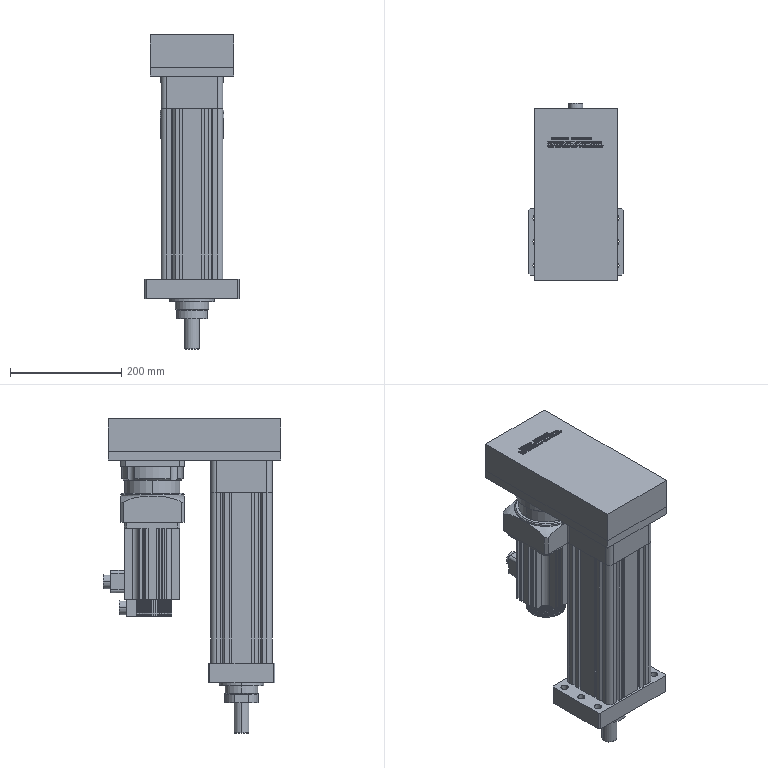Part | STEP file | 001-009-Servo press cylinder 5T-RKF120-150-P_RKF120-150-P | 7 solids | 3226 faces | volume 8858233 mm3 | plane 2230 | spline 765 | cylinder 216 | cone 15 | commonest cylinder face diameters 65 x50 1 x49 9 x16 20 x16 13 x12 8.7 x8